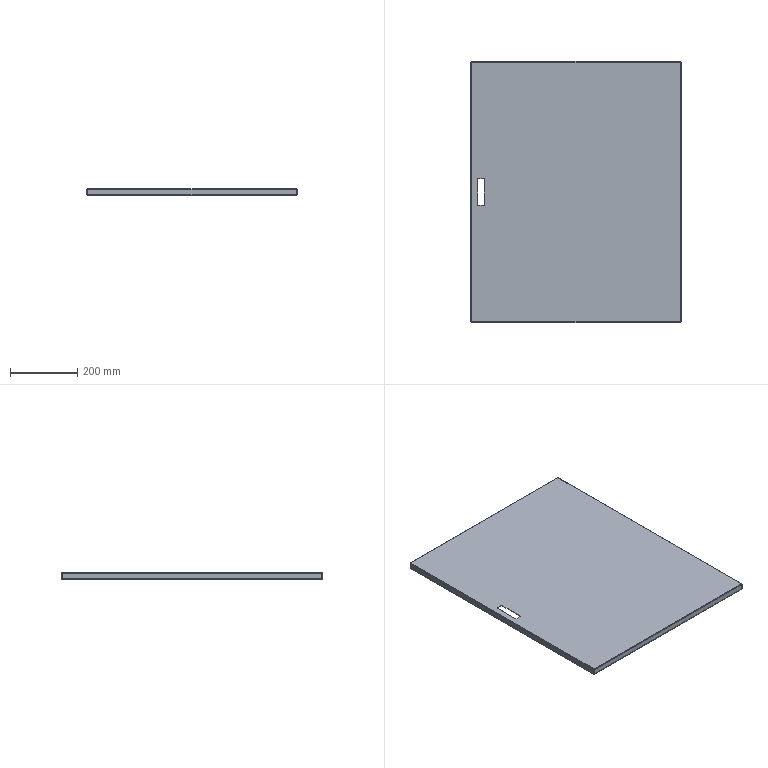Part | STEP file | X77-03018 | 1 solid | 74 faces | box 626 x 778 x 20 mm | volume 835340 mm3 | plane 42 | spline 16 | cylinder 16 | commonest cylinder face diameters 1.473 x8 4.473 x8